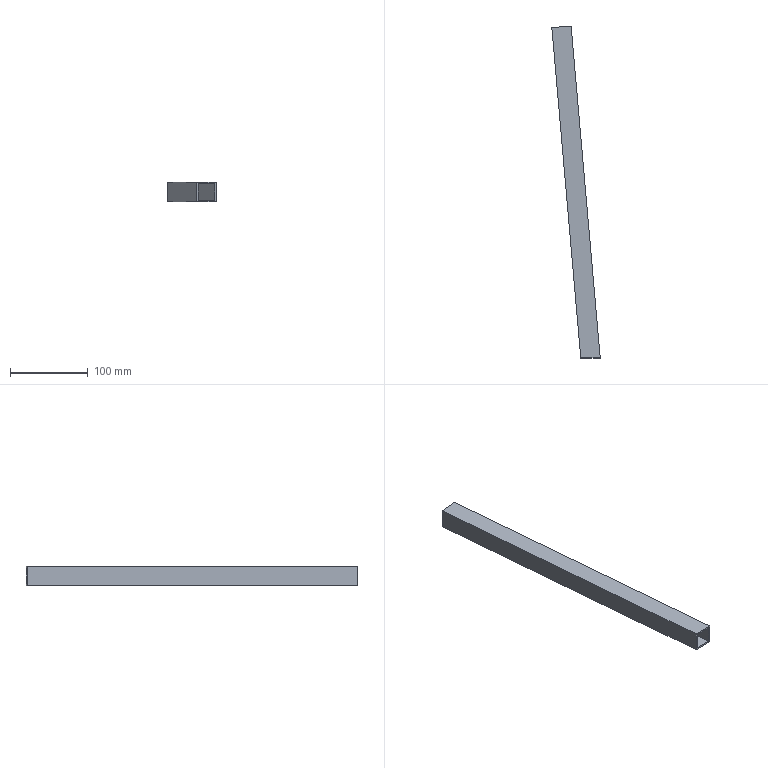Part | NX | features solid 2 | 1 solid | 10 faces | box 62.355 x 428.062 x 25 mm | volume 78863 mm3 | plane 10
STEP:
#1=CARTESIAN_POINT('',(552.959,313.383,-30.));
#2=VERTEX_POINT('',#1);
#3=CARTESIAN_POINT('',(552.959,313.383,-5.));
#4=VERTEX_POINT('',#3);
#5=CARTESIAN_POINT('',(552.959,313.383,-30.));
#6=DIRECTION('',(0.,0.,-1.));
#7=VECTOR('',#6,1000.);
#8=LINE('',#5,#7);
#9=EDGE_CURVE('',#2,#4,#8,.F.);
#10=ORIENTED_EDGE('',*,*,#9,.T.);
#11=CARTESIAN_POINT('',(577.864,315.562,-5.));
#12=VERTEX_POINT('',#11);
#13=CARTESIAN_POINT('',(552.959,313.383,-5.));
#14=DIRECTION('',(0.9962,0.08716,0.));
#15=VECTOR('',#14,1000.);
#16=LINE('',#13,#15);
#17=EDGE_CURVE('',#4,#12,#16,.T.);
#18=ORIENTED_EDGE('',*,*,#17,.T.);
#19=CARTESIAN_POINT('',(577.864,315.562,-30.));
#20=VERTEX_POINT('',#19);
#21=CARTESIAN_POINT('',(577.864,315.562,-30.));
#22=DIRECTION('',(0.,0.,-1.));
#23=VECTOR('',#22,1000.);
#24=LINE('',#21,#23);
#25=EDGE_CURVE('',#20,#12,#24,.F.);
#26=ORIENTED_EDGE('',*,*,#25,.F.);
#27=CARTESIAN_POINT('',(552.959,313.383,-30.));
#28=DIRECTION('',(-0.9962,-0.08716,0.));
#29=VECTOR('',#28,1000.);
#30=LINE('',#27,#29);
#31=EDGE_CURVE('',#2,#20,#30,.F.);
#32=ORIENTED_EDGE('',*,*,#31,.F.);
#33=EDGE_LOOP('',(#10,#18,#26,#32));
#34=FACE_BOUND('',#33,.T.);
#35=CARTESIAN_POINT('',(554.951,313.557,-28.));
#36=VERTEX_POINT('',#35);
#37=CARTESIAN_POINT('',(575.871,315.387,-28.));
#38=VERTEX_POINT('',#37);
#39=CARTESIAN_POINT('',(552.959,313.383,-28.));
#40=DIRECTION('',(-0.9962,-0.08716,0.));
#41=VECTOR('',#40,1000.);
#42=LINE('',#39,#41);
#43=EDGE_CURVE('',#36,#38,#42,.F.);
#44=ORIENTED_EDGE('',*,*,#43,.T.);
#45=CARTESIAN_POINT('',(575.871,315.387,-7.));
#46=VERTEX_POINT('',#45);
#47=CARTESIAN_POINT('',(575.871,315.387,-30.));
#48=DIRECTION('',(0.,0.,-1.));
#49=VECTOR('',#48,1000.);
#50=LINE('',#47,#49);
#51=EDGE_CURVE('',#38,#46,#50,.F.);
#52=ORIENTED_EDGE('',*,*,#51,.T.);
#53=CARTESIAN_POINT('',(554.951,313.557,-7.));
#54=VERTEX_POINT('',#53);
#55=CARTESIAN_POINT('',(552.959,313.383,-7.));
#56=DIRECTION('',(0.9962,0.08716,0.));
#57=VECTOR('',#56,1000.);
#58=LINE('',#55,#57);
#59=EDGE_CURVE('',#54,#46,#58,.T.);
#60=ORIENTED_EDGE('',*,*,#59,.F.);
#61=CARTESIAN_POINT('',(554.951,313.557,-30.));
#62=DIRECTION('',(0.,0.,-1.));
#63=VECTOR('',#62,1000.);
#64=LINE('',#61,#63);
#65=EDGE_CURVE('',#36,#54,#64,.F.);
#66=ORIENTED_EDGE('',*,*,#65,.F.);
#67=EDGE_LOOP('',(#44,#52,#60,#66));
#68=FACE_BOUND('',#67,.T.);
#69=CARTESIAN_POINT('',(552.959,313.383,-30.));
#70=DIRECTION('',(0.08716,-0.9962,0.));
#71=DIRECTION('',(0.,0.,1.));
#72=AXIS2_PLACEMENT_3D('',#69,#70,#71);
#73=PLANE('',#72);
#74=ADVANCED_FACE('',(#34,#68),#73,.F.);
#75=ORIENTED_EDGE('',*,*,#31,.T.);
#76=CARTESIAN_POINT('',(615.314,-112.5,-30.));
#77=VERTEX_POINT('',#76);
#78=CARTESIAN_POINT('',(612.726,-82.916,-30.));
#79=DIRECTION('',(-0.08716,0.9962,0.));
#80=VECTOR('',#79,1000.);
#81=LINE('',#78,#80);
#82=EDGE_CURVE('',#20,#77,#81,.F.);
#83=ORIENTED_EDGE('',*,*,#82,.T.);
#84=CARTESIAN_POINT('',(590.219,-112.5,-30.));
#85=VERTEX_POINT('',#84);
#86=CARTESIAN_POINT('',(587.821,-112.5,-30.));
#87=DIRECTION('',(-1.,0.,0.));
#88=VECTOR('',#87,1000.);
#89=LINE('',#86,#88);
#90=EDGE_CURVE('',#85,#77,#89,.F.);
#91=ORIENTED_EDGE('',*,*,#90,.F.);
#92=CARTESIAN_POINT('',(587.821,-85.095,-30.));
#93=DIRECTION('',(0.08716,-0.9962,0.));
#94=VECTOR('',#93,1000.);
#95=LINE('',#92,#94);
#96=EDGE_CURVE('',#2,#85,#95,.T.);
#97=ORIENTED_EDGE('',*,*,#96,.F.);
#98=EDGE_LOOP('',(#75,#83,#91,#97));
#99=FACE_BOUND('',#98,.T.);
#100=CARTESIAN_POINT('',(587.821,-85.095,-30.));
#101=DIRECTION('',(0.,0.,-1.));
#102=DIRECTION('',(0.08716,-0.9962,0.));
#103=AXIS2_PLACEMENT_3D('',#100,#101,#102);
#104=PLANE('',#103);
#105=ADVANCED_FACE('',(#99),#104,.T.);
#106=CARTESIAN_POINT('',(613.307,-112.5,-28.));
#107=VERTEX_POINT('',#106);
#108=CARTESIAN_POINT('',(592.226,-112.5,-28.));
#109=VERTEX_POINT('',#108);
#110=CARTESIAN_POINT('',(690.,-112.5,-28.));
#111=DIRECTION('',(1.,0.,0.));
#112=VECTOR('',#111,1000.);
#113=LINE('',#110,#112);
#114=EDGE_CURVE('',#107,#109,#113,.F.);
#115=ORIENTED_EDGE('',*,*,#114,.T.);
#116=CARTESIAN_POINT('',(592.226,-112.5,-7.));
#117=VERTEX_POINT('',#116);
#118=CARTESIAN_POINT('',(592.226,-112.5,-55.));
#119=DIRECTION('',(0.,0.,1.));
#120=VECTOR('',#119,1000.);
#121=LINE('',#118,#120);
#122=EDGE_CURVE('',#117,#109,#121,.F.);
#123=ORIENTED_EDGE('',*,*,#122,.F.);
#124=CARTESIAN_POINT('',(613.307,-112.5,-7.));
#125=VERTEX_POINT('',#124);
#126=CARTESIAN_POINT('',(690.,-112.5,-7.));
#127=DIRECTION('',(1.,0.,0.));
#128=VECTOR('',#127,1000.);
#129=LINE('',#126,#128);
#130=EDGE_CURVE('',#125,#117,#129,.F.);
#131=ORIENTED_EDGE('',*,*,#130,.F.);
#132=CARTESIAN_POINT('',(613.307,-112.5,-55.));
#133=DIRECTION('',(0.,0.,1.));
#134=VECTOR('',#133,1000.);
#135=LINE('',#132,#134);
#136=EDGE_CURVE('',#125,#107,#135,.F.);
#137=ORIENTED_EDGE('',*,*,#136,.T.);
#138=EDGE_LOOP('',(#115,#123,#131,#137));
#139=FACE_BOUND('',#138,.T.);
#140=ORIENTED_EDGE('',*,*,#90,.T.);
#141=CARTESIAN_POINT('',(615.314,-112.5,-5.));
#142=VERTEX_POINT('',#141);
#143=CARTESIAN_POINT('',(615.314,-112.5,-30.));
#144=DIRECTION('',(0.,0.,-1.));
#145=VECTOR('',#144,1000.);
#146=LINE('',#143,#145);
#147=EDGE_CURVE('',#77,#142,#146,.F.);
#148=ORIENTED_EDGE('',*,*,#147,.T.);
#149=CARTESIAN_POINT('',(590.219,-112.5,-5.));
#150=VERTEX_POINT('',#149);
#151=CARTESIAN_POINT('',(690.,-112.5,-5.));
#152=DIRECTION('',(1.,0.,0.));
#153=VECTOR('',#152,1000.);
#154=LINE('',#151,#153);
#155=EDGE_CURVE('',#150,#142,#154,.T.);
#156=ORIENTED_EDGE('',*,*,#155,.F.);
#157=CARTESIAN_POINT('',(590.219,-112.5,-30.));
#158=DIRECTION('',(0.,0.,-1.));
#159=VECTOR('',#158,1000.);
#160=LINE('',#157,#159);
#161=EDGE_CURVE('',#85,#150,#160,.F.);
#162=ORIENTED_EDGE('',*,*,#161,.F.);
#163=EDGE_LOOP('',(#140,#148,#156,#162));
#164=FACE_BOUND('',#163,.T.);
#165=CARTESIAN_POINT('',(690.,-112.5,-55.));
#166=DIRECTION('',(0.,1.,0.));
#167=DIRECTION('',(-1.,0.,0.));
#168=AXIS2_PLACEMENT_3D('',#165,#166,#167);
#169=PLANE('',#168);
#170=ADVANCED_FACE('',(#139,#164),#169,.F.);
#171=ORIENTED_EDGE('',*,*,#155,.T.);
#172=CARTESIAN_POINT('',(612.726,-82.916,-5.));
#173=DIRECTION('',(-0.08716,0.9962,0.));
#174=VECTOR('',#173,1000.);
#175=LINE('',#172,#174);
#176=EDGE_CURVE('',#12,#142,#175,.F.);
#177=ORIENTED_EDGE('',*,*,#176,.F.);
#178=ORIENTED_EDGE('',*,*,#17,.F.);
#179=CARTESIAN_POINT('',(587.821,-85.095,-5.));
#180=DIRECTION('',(0.08716,-0.9962,0.));
#181=VECTOR('',#180,1000.);
#182=LINE('',#179,#181);
#183=EDGE_CURVE('',#4,#150,#182,.T.);
#184=ORIENTED_EDGE('',*,*,#183,.T.);
#185=EDGE_LOOP('',(#171,#177,#178,#184));
#186=FACE_BOUND('',#185,.T.);
#187=CARTESIAN_POINT('',(587.821,-85.095,-5.));
#188=DIRECTION('',(0.,0.,-1.));
#189=DIRECTION('',(0.08716,-0.9962,0.));
#190=AXIS2_PLACEMENT_3D('',#187,#188,#189);
#191=PLANE('',#190);
#192=ADVANCED_FACE('',(#186),#191,.F.);
#193=ORIENTED_EDGE('',*,*,#176,.T.);
#194=ORIENTED_EDGE('',*,*,#147,.F.);
#195=ORIENTED_EDGE('',*,*,#82,.F.);
#196=ORIENTED_EDGE('',*,*,#25,.T.);
#197=EDGE_LOOP('',(#193,#194,#195,#196));
#198=FACE_BOUND('',#197,.T.);
#199=CARTESIAN_POINT('',(612.726,-82.916,-30.));
#200=DIRECTION('',(0.9962,0.08716,0.));
#201=DIRECTION('',(0.,0.,1.));
#202=AXIS2_PLACEMENT_3D('',#199,#200,#201);
#203=PLANE('',#202);
#204=ADVANCED_FACE('',(#198),#203,.T.);
#205=ORIENTED_EDGE('',*,*,#183,.F.);
#206=ORIENTED_EDGE('',*,*,#9,.F.);
#207=ORIENTED_EDGE('',*,*,#96,.T.);
#208=ORIENTED_EDGE('',*,*,#161,.T.);
#209=EDGE_LOOP('',(#205,#206,#207,#208));
#210=FACE_BOUND('',#209,.T.);
#211=CARTESIAN_POINT('',(587.821,-85.095,-30.));
#212=DIRECTION('',(0.9962,0.08716,0.));
#213=DIRECTION('',(0.,0.,1.));
#214=AXIS2_PLACEMENT_3D('',#211,#212,#213);
#215=PLANE('',#214);
#216=ADVANCED_FACE('',(#210),#215,.F.);
#217=ORIENTED_EDGE('',*,*,#114,.F.);
#218=CARTESIAN_POINT('',(610.734,-83.091,-28.));
#219=DIRECTION('',(0.08716,-0.9962,0.));
#220=VECTOR('',#219,1000.);
#221=LINE('',#218,#220);
#222=EDGE_CURVE('',#38,#107,#221,.T.);
#223=ORIENTED_EDGE('',*,*,#222,.F.);
#224=ORIENTED_EDGE('',*,*,#43,.F.);
#225=CARTESIAN_POINT('',(589.813,-84.921,-28.));
#226=DIRECTION('',(0.08716,-0.9962,0.));
#227=VECTOR('',#226,1000.);
#228=LINE('',#225,#227);
#229=EDGE_CURVE('',#36,#109,#228,.T.);
#230=ORIENTED_EDGE('',*,*,#229,.T.);
#231=EDGE_LOOP('',(#217,#223,#224,#230));
#232=FACE_BOUND('',#231,.T.);
#233=CARTESIAN_POINT('',(587.821,-85.095,-28.));
#234=DIRECTION('',(0.,0.,-1.));
#235=DIRECTION('',(0.08716,-0.9962,0.));
#236=AXIS2_PLACEMENT_3D('',#233,#234,#235);
#237=PLANE('',#236);
#238=ADVANCED_FACE('',(#232),#237,.F.);
#239=ORIENTED_EDGE('',*,*,#130,.T.);
#240=CARTESIAN_POINT('',(589.813,-84.921,-7.));
#241=DIRECTION('',(-0.08716,0.9962,0.));
#242=VECTOR('',#241,1000.);
#243=LINE('',#240,#242);
#244=EDGE_CURVE('',#54,#117,#243,.F.);
#245=ORIENTED_EDGE('',*,*,#244,.F.);
#246=ORIENTED_EDGE('',*,*,#59,.T.);
#247=CARTESIAN_POINT('',(610.734,-83.091,-7.));
#248=DIRECTION('',(-0.08716,0.9962,0.));
#249=VECTOR('',#248,1000.);
#250=LINE('',#247,#249);
#251=EDGE_CURVE('',#46,#125,#250,.F.);
#252=ORIENTED_EDGE('',*,*,#251,.T.);
#253=EDGE_LOOP('',(#239,#245,#246,#252));
#254=FACE_BOUND('',#253,.T.);
#255=CARTESIAN_POINT('',(587.821,-85.095,-7.));
#256=DIRECTION('',(0.,0.,-1.));
#257=DIRECTION('',(0.08716,-0.9962,0.));
#258=AXIS2_PLACEMENT_3D('',#255,#256,#257);
#259=PLANE('',#258);
#260=ADVANCED_FACE('',(#254),#259,.T.);
#261=ORIENTED_EDGE('',*,*,#136,.F.);
#262=ORIENTED_EDGE('',*,*,#251,.F.);
#263=ORIENTED_EDGE('',*,*,#51,.F.);
#264=ORIENTED_EDGE('',*,*,#222,.T.);
#265=EDGE_LOOP('',(#261,#262,#263,#264));
#266=FACE_BOUND('',#265,.T.);
#267=CARTESIAN_POINT('',(610.734,-83.091,-30.));
#268=DIRECTION('',(0.9962,0.08716,0.));
#269=DIRECTION('',(0.,0.,1.));
#270=AXIS2_PLACEMENT_3D('',#267,#268,#269);
#271=PLANE('',#270);
#272=ADVANCED_FACE('',(#266),#271,.F.);
#273=ORIENTED_EDGE('',*,*,#122,.T.);
#274=ORIENTED_EDGE('',*,*,#229,.F.);
#275=ORIENTED_EDGE('',*,*,#65,.T.);
#276=ORIENTED_EDGE('',*,*,#244,.T.);
#277=EDGE_LOOP('',(#273,#274,#275,#276));
#278=FACE_BOUND('',#277,.T.);
#279=CARTESIAN_POINT('',(589.813,-84.921,-30.));
#280=DIRECTION('',(0.9962,0.08716,0.));
#281=DIRECTION('',(0.,0.,1.));
#282=AXIS2_PLACEMENT_3D('',#279,#280,#281);
#283=PLANE('',#282);
#284=ADVANCED_FACE('',(#278),#283,.T.);
#285=CLOSED_SHELL('',(#74,#105,#170,#192,#204,#216,#238,#260,#272,#284));
#286=MANIFOLD_SOLID_BREP('',#285);
#287=(LENGTH_UNIT()NAMED_UNIT(*)SI_UNIT(.MILLI.,.METRE.));
#288=UNCERTAINTY_MEASURE_WITH_UNIT(LENGTH_MEASURE(0.00001),#287,'','');
#289=(NAMED_UNIT(*)PLANE_ANGLE_UNIT()SI_UNIT($,.RADIAN.));
#290=(NAMED_UNIT(*)SI_UNIT($,.STERADIAN.)SOLID_ANGLE_UNIT());
#291=(GEOMETRIC_REPRESENTATION_CONTEXT(3)GLOBAL_UNCERTAINTY_ASSIGNED_CONTEXT((#288))GLOBAL_UNIT_ASSIGNED_CONTEXT((#287,#289,#290))REPRESENTATION_CONTEXT('',''));
#292=ADVANCED_BREP_SHAPE_REPRESENTATION('',(#286),#291);